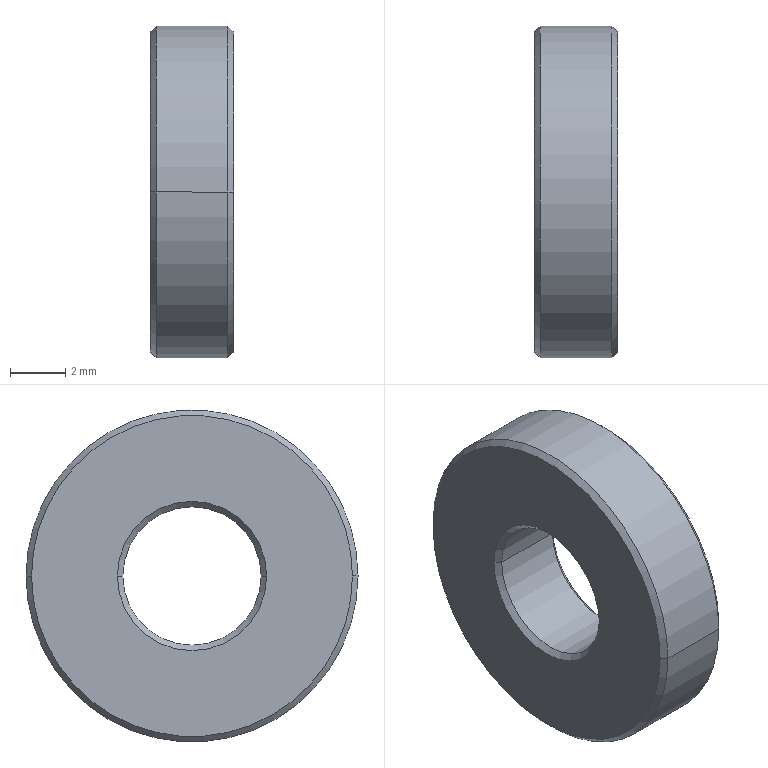Part | STEP file | WSSS12-5-3-16 | 1 solid | 14 faces | box 3 x 12 x 12 mm | volume 278.251 mm3 | cone 8 | cylinder 4 | plane 2 | commonest cylinder face diameters 5 x2 12 x2
STEP:
#1=CARTESIAN_POINT('',(0.,0.,0.));
#2=DIRECTION('',(0.,0.,1.));
#3=DIRECTION('',(1.,0.,0.));
#4=AXIS2_PLACEMENT_3D('',#1,#2,#3);
#5=CARTESIAN_POINT('',(2.8,-2.5,0.));
#6=VERTEX_POINT('',#5);
#7=CARTESIAN_POINT('',(0.2,-2.5,0.));
#8=VERTEX_POINT('',#7);
#9=CARTESIAN_POINT('',(-3.,-2.5,0.));
#10=DIRECTION('',(-1.,0.,0.));
#11=VECTOR('',#10,1.);
#12=LINE('',#9,#11);
#13=CARTESIAN_POINT('',(-3.,0.,0.));
#14=DIRECTION('',(-1.,0.,0.));
#15=DIRECTION('',(0.,-1.,0.));
#16=AXIS2_PLACEMENT_3D('',#13,#14,#15);
#17=CYLINDRICAL_SURFACE('',#16,2.5);
#18=CARTESIAN_POINT('',(6.283,0.));
#19=DIRECTION('',(0.,1.));
#20=VECTOR('',#19,1.);
#21=LINE('',#18,#20);
#22=(GEOMETRIC_REPRESENTATION_CONTEXT(2)PARAMETRIC_REPRESENTATION_CONTEXT()REPRESENTATION_CONTEXT('',''));
#23=DEFINITIONAL_REPRESENTATION('',(#21),#22);
#24=PCURVE('',#17,#23);
#25=CARTESIAN_POINT('',(-3.,0.,0.));
#26=DIRECTION('',(-1.,0.,0.));
#27=DIRECTION('',(0.,-1.,0.));
#28=AXIS2_PLACEMENT_3D('',#25,#26,#27);
#29=CYLINDRICAL_SURFACE('',#28,2.5);
#30=CARTESIAN_POINT('',(0.,0.));
#31=DIRECTION('',(0.,1.));
#32=VECTOR('',#31,1.);
#33=LINE('',#30,#32);
#34=(GEOMETRIC_REPRESENTATION_CONTEXT(2)PARAMETRIC_REPRESENTATION_CONTEXT()REPRESENTATION_CONTEXT('',''));
#35=DEFINITIONAL_REPRESENTATION('',(#33),#34);
#36=PCURVE('',#29,#35);
#37=SURFACE_CURVE('',#12,(#24,#36),.PCURVE_S1.);
#38=EDGE_CURVE('',#6,#8,#37,.T.);
#39=ORIENTED_EDGE('',*,*,#38,.T.);
#40=CARTESIAN_POINT('',(0.2,2.5,0.));
#41=VERTEX_POINT('',#40);
#42=CARTESIAN_POINT('',(0.2,0.,0.));
#43=DIRECTION('',(-1.,0.,0.));
#44=DIRECTION('',(0.,-1.,0.));
#45=AXIS2_PLACEMENT_3D('',#42,#43,#44);
#46=CIRCLE('',#45,2.5);
#47=CARTESIAN_POINT('',(0.,-3.2));
#48=DIRECTION('',(1.,0.));
#49=VECTOR('',#48,1.);
#50=LINE('',#47,#49);
#51=(GEOMETRIC_REPRESENTATION_CONTEXT(2)PARAMETRIC_REPRESENTATION_CONTEXT()REPRESENTATION_CONTEXT('',''));
#52=DEFINITIONAL_REPRESENTATION('',(#50),#51);
#53=PCURVE('',#17,#52);
#54=CARTESIAN_POINT('',(0.2,0.,0.));
#55=DIRECTION('',(-1.,0.,0.));
#56=DIRECTION('',(0.,-1.,0.));
#57=AXIS2_PLACEMENT_3D('',#54,#55,#56);
#58=CONICAL_SURFACE('',#57,2.5,0.7854);
#59=CARTESIAN_POINT('',(0.,0.));
#60=DIRECTION('',(1.,0.));
#61=VECTOR('',#60,1.);
#62=LINE('',#59,#61);
#63=(GEOMETRIC_REPRESENTATION_CONTEXT(2)PARAMETRIC_REPRESENTATION_CONTEXT()REPRESENTATION_CONTEXT('',''));
#64=DEFINITIONAL_REPRESENTATION('',(#62),#63);
#65=PCURVE('',#58,#64);
#66=SURFACE_CURVE('',#46,(#53,#65),.PCURVE_S1.);
#67=EDGE_CURVE('',#41,#8,#66,.T.);
#68=ORIENTED_EDGE('',*,*,#67,.F.);
#69=CARTESIAN_POINT('',(2.8,2.5,0.));
#70=VERTEX_POINT('',#69);
#71=CARTESIAN_POINT('',(-3.,2.5,0.));
#72=DIRECTION('',(-1.,0.,0.));
#73=VECTOR('',#72,1.);
#74=LINE('',#71,#73);
#75=CARTESIAN_POINT('',(3.142,0.));
#76=DIRECTION('',(0.,1.));
#77=VECTOR('',#76,1.);
#78=LINE('',#75,#77);
#79=(GEOMETRIC_REPRESENTATION_CONTEXT(2)PARAMETRIC_REPRESENTATION_CONTEXT()REPRESENTATION_CONTEXT('',''));
#80=DEFINITIONAL_REPRESENTATION('',(#78),#79);
#81=PCURVE('',#17,#80);
#82=CARTESIAN_POINT('',(3.142,0.));
#83=DIRECTION('',(0.,1.));
#84=VECTOR('',#83,1.);
#85=LINE('',#82,#84);
#86=(GEOMETRIC_REPRESENTATION_CONTEXT(2)PARAMETRIC_REPRESENTATION_CONTEXT()REPRESENTATION_CONTEXT('',''));
#87=DEFINITIONAL_REPRESENTATION('',(#85),#86);
#88=PCURVE('',#29,#87);
#89=SURFACE_CURVE('',#74,(#81,#88),.PCURVE_S1.);
#90=EDGE_CURVE('',#70,#41,#89,.T.);
#91=ORIENTED_EDGE('',*,*,#90,.F.);
#92=CARTESIAN_POINT('',(2.8,0.,0.));
#93=DIRECTION('',(-1.,0.,0.));
#94=DIRECTION('',(0.,-1.,0.));
#95=AXIS2_PLACEMENT_3D('',#92,#93,#94);
#96=CIRCLE('',#95,2.5);
#97=CARTESIAN_POINT('',(0.,-5.8));
#98=DIRECTION('',(1.,0.));
#99=VECTOR('',#98,1.);
#100=LINE('',#97,#99);
#101=(GEOMETRIC_REPRESENTATION_CONTEXT(2)PARAMETRIC_REPRESENTATION_CONTEXT()REPRESENTATION_CONTEXT('',''));
#102=DEFINITIONAL_REPRESENTATION('',(#100),#101);
#103=PCURVE('',#17,#102);
#104=CARTESIAN_POINT('',(3.,0.,0.));
#105=DIRECTION('',(1.,0.,0.));
#106=DIRECTION('',(0.,1.,0.));
#107=AXIS2_PLACEMENT_3D('',#104,#105,#106);
#108=CONICAL_SURFACE('',#107,2.7,0.7854);
#109=CARTESIAN_POINT('',(9.425,-0.2));
#110=DIRECTION('',(-1.,0.));
#111=VECTOR('',#110,1.);
#112=LINE('',#109,#111);
#113=(GEOMETRIC_REPRESENTATION_CONTEXT(2)PARAMETRIC_REPRESENTATION_CONTEXT()REPRESENTATION_CONTEXT('',''));
#114=DEFINITIONAL_REPRESENTATION('',(#112),#113);
#115=PCURVE('',#108,#114);
#116=SURFACE_CURVE('',#96,(#103,#115),.PCURVE_S1.);
#117=EDGE_CURVE('',#70,#6,#116,.T.);
#118=ORIENTED_EDGE('',*,*,#117,.T.);
#119=EDGE_LOOP('',(#39,#68,#91,#118));
#120=FACE_BOUND('',#119,.F.);
#121=ADVANCED_FACE('',(#120),#17,.F.);
#122=CARTESIAN_POINT('',(3.,2.7,0.));
#123=VERTEX_POINT('',#122);
#124=CARTESIAN_POINT('',(3.,2.7,0.));
#125=DIRECTION('',(0.7071,0.7071,0.));
#126=VECTOR('',#125,1.);
#127=LINE('',#124,#126);
#128=CARTESIAN_POINT('',(6.283,0.));
#129=DIRECTION('',(0.,1.));
#130=VECTOR('',#129,1.);
#131=LINE('',#128,#130);
#132=(GEOMETRIC_REPRESENTATION_CONTEXT(2)PARAMETRIC_REPRESENTATION_CONTEXT()REPRESENTATION_CONTEXT('',''));
#133=DEFINITIONAL_REPRESENTATION('',(#131),#132);
#134=PCURVE('',#108,#133);
#135=CARTESIAN_POINT('',(3.,0.,0.));
#136=DIRECTION('',(1.,0.,0.));
#137=DIRECTION('',(0.,1.,0.));
#138=AXIS2_PLACEMENT_3D('',#135,#136,#137);
#139=CONICAL_SURFACE('',#138,2.7,0.7854);
#140=CARTESIAN_POINT('',(0.,0.));
#141=DIRECTION('',(0.,1.));
#142=VECTOR('',#141,1.);
#143=LINE('',#140,#142);
#144=(GEOMETRIC_REPRESENTATION_CONTEXT(2)PARAMETRIC_REPRESENTATION_CONTEXT()REPRESENTATION_CONTEXT('',''));
#145=DEFINITIONAL_REPRESENTATION('',(#143),#144);
#146=PCURVE('',#139,#145);
#147=SURFACE_CURVE('',#127,(#134,#146),.PCURVE_S1.);
#148=EDGE_CURVE('',#70,#123,#147,.T.);
#149=ORIENTED_EDGE('',*,*,#148,.T.);
#150=CARTESIAN_POINT('',(3.,-2.7,0.));
#151=VERTEX_POINT('',#150);
#152=CARTESIAN_POINT('',(3.,0.,0.));
#153=DIRECTION('',(-1.,0.,0.));
#154=DIRECTION('',(0.,-1.,0.));
#155=AXIS2_PLACEMENT_3D('',#152,#153,#154);
#156=CIRCLE('',#155,2.7);
#157=CARTESIAN_POINT('',(9.425,0.));
#158=DIRECTION('',(-1.,0.));
#159=VECTOR('',#158,1.);
#160=LINE('',#157,#159);
#161=(GEOMETRIC_REPRESENTATION_CONTEXT(2)PARAMETRIC_REPRESENTATION_CONTEXT()REPRESENTATION_CONTEXT('',''));
#162=DEFINITIONAL_REPRESENTATION('',(#160),#161);
#163=PCURVE('',#108,#162);
#164=CARTESIAN_POINT('',(3.,-6.8,0.));
#165=DIRECTION('',(1.,0.,0.));
#166=DIRECTION('',(0.,1.,0.));
#167=AXIS2_PLACEMENT_3D('',#164,#165,#166);
#168=PLANE('',#167);
#169=CARTESIAN_POINT('',(4.1,0.));
#170=CARTESIAN_POINT('',(4.1,4.677));
#171=CARTESIAN_POINT('',(8.15,2.338));
#172=CARTESIAN_POINT('',(12.2,0.));
#173=CARTESIAN_POINT('',(8.15,-2.338));
#174=CARTESIAN_POINT('',(4.1,-4.677));
#175=CARTESIAN_POINT('',(4.1,0.));
#176=(BOUNDED_CURVE()B_SPLINE_CURVE(2,(#169,#170,#171,#172,#173,#174,#175),.UNSPECIFIED.,.T.,.F.)B_SPLINE_CURVE_WITH_KNOTS((1,2,2,2,2,1),(-2.094,0.,2.094,4.189,6.283,8.378),.UNSPECIFIED.)CURVE()GEOMETRIC_REPRESENTATION_ITEM()RATIONAL_B_SPLINE_CURVE((1.,0.5,1.,0.5,1.,0.5,1.))REPRESENTATION_ITEM(''));
#177=(GEOMETRIC_REPRESENTATION_CONTEXT(2)PARAMETRIC_REPRESENTATION_CONTEXT()REPRESENTATION_CONTEXT('',''));
#178=DEFINITIONAL_REPRESENTATION('',(#176),#177);
#179=PCURVE('',#168,#178);
#180=SURFACE_CURVE('',#156,(#163,#179),.PCURVE_S1.);
#181=EDGE_CURVE('',#123,#151,#180,.T.);
#182=ORIENTED_EDGE('',*,*,#181,.T.);
#183=CARTESIAN_POINT('',(3.,-2.7,0.));
#184=DIRECTION('',(0.7071,-0.7071,0.));
#185=VECTOR('',#184,1.);
#186=LINE('',#183,#185);
#187=CARTESIAN_POINT('',(3.142,0.));
#188=DIRECTION('',(0.,1.));
#189=VECTOR('',#188,1.);
#190=LINE('',#187,#189);
#191=(GEOMETRIC_REPRESENTATION_CONTEXT(2)PARAMETRIC_REPRESENTATION_CONTEXT()REPRESENTATION_CONTEXT('',''));
#192=DEFINITIONAL_REPRESENTATION('',(#190),#191);
#193=PCURVE('',#108,#192);
#194=CARTESIAN_POINT('',(3.142,0.));
#195=DIRECTION('',(0.,1.));
#196=VECTOR('',#195,1.);
#197=LINE('',#194,#196);
#198=(GEOMETRIC_REPRESENTATION_CONTEXT(2)PARAMETRIC_REPRESENTATION_CONTEXT()REPRESENTATION_CONTEXT('',''));
#199=DEFINITIONAL_REPRESENTATION('',(#197),#198);
#200=PCURVE('',#139,#199);
#201=SURFACE_CURVE('',#186,(#193,#200),.PCURVE_S1.);
#202=EDGE_CURVE('',#6,#151,#201,.T.);
#203=ORIENTED_EDGE('',*,*,#202,.F.);
#204=ORIENTED_EDGE('',*,*,#117,.F.);
#205=EDGE_LOOP('',(#149,#182,#203,#204));
#206=FACE_BOUND('',#205,.F.);
#207=ADVANCED_FACE('',(#206),#108,.F.);
#208=CARTESIAN_POINT('',(3.,-5.8,0.));
#209=VERTEX_POINT('',#208);
#210=CARTESIAN_POINT('',(3.,5.8,0.));
#211=VERTEX_POINT('',#210);
#212=CARTESIAN_POINT('',(3.,0.,0.));
#213=DIRECTION('',(-1.,0.,0.));
#214=DIRECTION('',(0.,1.,0.));
#215=AXIS2_PLACEMENT_3D('',#212,#213,#214);
#216=CIRCLE('',#215,5.8);
#217=CARTESIAN_POINT('',(2.8,0.,0.));
#218=DIRECTION('',(-1.,0.,0.));
#219=DIRECTION('',(0.,-1.,0.));
#220=AXIS2_PLACEMENT_3D('',#217,#218,#219);
#221=CONICAL_SURFACE('',#220,6.,0.7854);
#222=CARTESIAN_POINT('',(-3.142,-0.2));
#223=DIRECTION('',(1.,0.));
#224=VECTOR('',#223,1.);
#225=LINE('',#222,#224);
#226=(GEOMETRIC_REPRESENTATION_CONTEXT(2)PARAMETRIC_REPRESENTATION_CONTEXT()REPRESENTATION_CONTEXT('',''));
#227=DEFINITIONAL_REPRESENTATION('',(#225),#226);
#228=PCURVE('',#221,#227);
#229=CARTESIAN_POINT('',(12.6,0.));
#230=CARTESIAN_POINT('',(12.6,-10.046));
#231=CARTESIAN_POINT('',(3.9,-5.023));
#232=CARTESIAN_POINT('',(-4.8,0.));
#233=CARTESIAN_POINT('',(3.9,5.023));
#234=CARTESIAN_POINT('',(12.6,10.046));
#235=CARTESIAN_POINT('',(12.6,0.));
#236=(BOUNDED_CURVE()B_SPLINE_CURVE(2,(#229,#230,#231,#232,#233,#234,#235),.UNSPECIFIED.,.T.,.F.)B_SPLINE_CURVE_WITH_KNOTS((1,2,2,2,2,1),(-2.094,0.,2.094,4.189,6.283,8.378),.UNSPECIFIED.)CURVE()GEOMETRIC_REPRESENTATION_ITEM()RATIONAL_B_SPLINE_CURVE((1.,0.5,1.,0.5,1.,0.5,1.))REPRESENTATION_ITEM(''));
#237=(GEOMETRIC_REPRESENTATION_CONTEXT(2)PARAMETRIC_REPRESENTATION_CONTEXT()REPRESENTATION_CONTEXT('',''));
#238=DEFINITIONAL_REPRESENTATION('',(#236),#237);
#239=PCURVE('',#168,#238);
#240=SURFACE_CURVE('',#216,(#228,#239),.PCURVE_S1.);
#241=EDGE_CURVE('',#209,#211,#240,.T.);
#242=ORIENTED_EDGE('',*,*,#241,.T.);
#243=CARTESIAN_POINT('',(2.8,6.,0.));
#244=VERTEX_POINT('',#243);
#245=CARTESIAN_POINT('',(2.8,6.,0.));
#246=DIRECTION('',(-0.7071,0.7071,0.));
#247=VECTOR('',#246,1.);
#248=LINE('',#245,#247);
#249=CARTESIAN_POINT('',(3.142,0.));
#250=DIRECTION('',(0.,1.));
#251=VECTOR('',#250,1.);
#252=LINE('',#249,#251);
#253=(GEOMETRIC_REPRESENTATION_CONTEXT(2)PARAMETRIC_REPRESENTATION_CONTEXT()REPRESENTATION_CONTEXT('',''));
#254=DEFINITIONAL_REPRESENTATION('',(#252),#253);
#255=PCURVE('',#221,#254);
#256=CARTESIAN_POINT('',(2.8,0.,0.));
#257=DIRECTION('',(-1.,0.,0.));
#258=DIRECTION('',(0.,-1.,0.));
#259=AXIS2_PLACEMENT_3D('',#256,#257,#258);
#260=CONICAL_SURFACE('',#259,6.,0.7854);
#261=CARTESIAN_POINT('',(3.142,0.));
#262=DIRECTION('',(0.,1.));
#263=VECTOR('',#262,1.);
#264=LINE('',#261,#263);
#265=(GEOMETRIC_REPRESENTATION_CONTEXT(2)PARAMETRIC_REPRESENTATION_CONTEXT()REPRESENTATION_CONTEXT('',''));
#266=DEFINITIONAL_REPRESENTATION('',(#264),#265);
#267=PCURVE('',#260,#266);
#268=SURFACE_CURVE('',#248,(#255,#267),.PCURVE_S1.);
#269=EDGE_CURVE('',#211,#244,#268,.T.);
#270=ORIENTED_EDGE('',*,*,#269,.T.);
#271=CARTESIAN_POINT('',(2.8,-6.,0.));
#272=VERTEX_POINT('',#271);
#273=CARTESIAN_POINT('',(2.8,0.,0.));
#274=DIRECTION('',(-1.,0.,0.));
#275=DIRECTION('',(0.,-1.,0.));
#276=AXIS2_PLACEMENT_3D('',#273,#274,#275);
#277=CIRCLE('',#276,6.);
#278=CARTESIAN_POINT('',(0.,0.));
#279=DIRECTION('',(1.,0.));
#280=VECTOR('',#279,1.);
#281=LINE('',#278,#280);
#282=(GEOMETRIC_REPRESENTATION_CONTEXT(2)PARAMETRIC_REPRESENTATION_CONTEXT()REPRESENTATION_CONTEXT('',''));
#283=DEFINITIONAL_REPRESENTATION('',(#281),#282);
#284=PCURVE('',#221,#283);
#285=CARTESIAN_POINT('',(-3.,0.,0.));
#286=DIRECTION('',(-1.,0.,0.));
#287=DIRECTION('',(0.,-1.,0.));
#288=AXIS2_PLACEMENT_3D('',#285,#286,#287);
#289=CYLINDRICAL_SURFACE('',#288,6.);
#290=CARTESIAN_POINT('',(0.,-5.8));
#291=DIRECTION('',(1.,0.));
#292=VECTOR('',#291,1.);
#293=LINE('',#290,#292);
#294=(GEOMETRIC_REPRESENTATION_CONTEXT(2)PARAMETRIC_REPRESENTATION_CONTEXT()REPRESENTATION_CONTEXT('',''));
#295=DEFINITIONAL_REPRESENTATION('',(#293),#294);
#296=PCURVE('',#289,#295);
#297=SURFACE_CURVE('',#277,(#284,#296),.PCURVE_S1.);
#298=EDGE_CURVE('',#272,#244,#297,.T.);
#299=ORIENTED_EDGE('',*,*,#298,.F.);
#300=CARTESIAN_POINT('',(2.8,-6.,0.));
#301=DIRECTION('',(-0.7071,-0.7071,0.));
#302=VECTOR('',#301,1.);
#303=LINE('',#300,#302);
#304=CARTESIAN_POINT('',(0.,0.));
#305=DIRECTION('',(0.,1.));
#306=VECTOR('',#305,1.);
#307=LINE('',#304,#306);
#308=(GEOMETRIC_REPRESENTATION_CONTEXT(2)PARAMETRIC_REPRESENTATION_CONTEXT()REPRESENTATION_CONTEXT('',''));
#309=DEFINITIONAL_REPRESENTATION('',(#307),#308);
#310=PCURVE('',#221,#309);
#311=CARTESIAN_POINT('',(6.283,0.));
#312=DIRECTION('',(0.,1.));
#313=VECTOR('',#312,1.);
#314=LINE('',#311,#313);
#315=(GEOMETRIC_REPRESENTATION_CONTEXT(2)PARAMETRIC_REPRESENTATION_CONTEXT()REPRESENTATION_CONTEXT('',''));
#316=DEFINITIONAL_REPRESENTATION('',(#314),#315);
#317=PCURVE('',#260,#316);
#318=SURFACE_CURVE('',#303,(#310,#317),.PCURVE_S1.);
#319=EDGE_CURVE('',#209,#272,#318,.T.);
#320=ORIENTED_EDGE('',*,*,#319,.F.);
#321=EDGE_LOOP('',(#242,#270,#299,#320));
#322=FACE_BOUND('',#321,.T.);
#323=ADVANCED_FACE('',(#322),#221,.T.);
#324=ORIENTED_EDGE('',*,*,#298,.T.);
#325=CARTESIAN_POINT('',(0.2,6.,0.));
#326=VERTEX_POINT('',#325);
#327=CARTESIAN_POINT('',(-3.,6.,0.));
#328=DIRECTION('',(-1.,0.,0.));
#329=VECTOR('',#328,1.);
#330=LINE('',#327,#329);
#331=CARTESIAN_POINT('',(3.142,0.));
#332=DIRECTION('',(0.,1.));
#333=VECTOR('',#332,1.);
#334=LINE('',#331,#333);
#335=(GEOMETRIC_REPRESENTATION_CONTEXT(2)PARAMETRIC_REPRESENTATION_CONTEXT()REPRESENTATION_CONTEXT('',''));
#336=DEFINITIONAL_REPRESENTATION('',(#334),#335);
#337=PCURVE('',#289,#336);
#338=CARTESIAN_POINT('',(-3.,0.,0.));
#339=DIRECTION('',(-1.,0.,0.));
#340=DIRECTION('',(0.,-1.,0.));
#341=AXIS2_PLACEMENT_3D('',#338,#339,#340);
#342=CYLINDRICAL_SURFACE('',#341,6.);
#343=CARTESIAN_POINT('',(3.142,0.));
#344=DIRECTION('',(0.,1.));
#345=VECTOR('',#344,1.);
#346=LINE('',#343,#345);
#347=(GEOMETRIC_REPRESENTATION_CONTEXT(2)PARAMETRIC_REPRESENTATION_CONTEXT()REPRESENTATION_CONTEXT('',''));
#348=DEFINITIONAL_REPRESENTATION('',(#346),#347);
#349=PCURVE('',#342,#348);
#350=SURFACE_CURVE('',#330,(#337,#349),.PCURVE_S1.);
#351=EDGE_CURVE('',#244,#326,#350,.T.);
#352=ORIENTED_EDGE('',*,*,#351,.T.);
#353=CARTESIAN_POINT('',(0.2,-6.,0.));
#354=VERTEX_POINT('',#353);
#355=CARTESIAN_POINT('',(0.2,0.,0.));
#356=DIRECTION('',(-1.,0.,0.));
#357=DIRECTION('',(0.,1.,0.));
#358=AXIS2_PLACEMENT_3D('',#355,#356,#357);
#359=CIRCLE('',#358,6.);
#360=CARTESIAN_POINT('',(-3.142,-3.2));
#361=DIRECTION('',(1.,0.));
#362=VECTOR('',#361,1.);
#363=LINE('',#360,#362);
#364=(GEOMETRIC_REPRESENTATION_CONTEXT(2)PARAMETRIC_REPRESENTATION_CONTEXT()REPRESENTATION_CONTEXT('',''));
#365=DEFINITIONAL_REPRESENTATION('',(#363),#364);
#366=PCURVE('',#289,#365);
#367=CARTESIAN_POINT('',(0.,0.,0.));
#368=DIRECTION('',(1.,0.,0.));
#369=DIRECTION('',(0.,1.,0.));
#370=AXIS2_PLACEMENT_3D('',#367,#368,#369);
#371=CONICAL_SURFACE('',#370,5.8,0.7854);
#372=CARTESIAN_POINT('',(6.283,0.2));
#373=DIRECTION('',(-1.,0.));
#374=VECTOR('',#373,1.);
#375=LINE('',#372,#374);
#376=(GEOMETRIC_REPRESENTATION_CONTEXT(2)PARAMETRIC_REPRESENTATION_CONTEXT()REPRESENTATION_CONTEXT('',''));
#377=DEFINITIONAL_REPRESENTATION('',(#375),#376);
#378=PCURVE('',#371,#377);
#379=SURFACE_CURVE('',#359,(#366,#378),.PCURVE_S1.);
#380=EDGE_CURVE('',#354,#326,#379,.T.);
#381=ORIENTED_EDGE('',*,*,#380,.F.);
#382=CARTESIAN_POINT('',(-3.,-6.,0.));
#383=DIRECTION('',(-1.,0.,0.));
#384=VECTOR('',#383,1.);
#385=LINE('',#382,#384);
#386=CARTESIAN_POINT('',(0.,0.));
#387=DIRECTION('',(0.,1.));
#388=VECTOR('',#387,1.);
#389=LINE('',#386,#388);
#390=(GEOMETRIC_REPRESENTATION_CONTEXT(2)PARAMETRIC_REPRESENTATION_CONTEXT()REPRESENTATION_CONTEXT('',''));
#391=DEFINITIONAL_REPRESENTATION('',(#389),#390);
#392=PCURVE('',#289,#391);
#393=CARTESIAN_POINT('',(6.283,0.));
#394=DIRECTION('',(0.,1.));
#395=VECTOR('',#394,1.);
#396=LINE('',#393,#395);
#397=(GEOMETRIC_REPRESENTATION_CONTEXT(2)PARAMETRIC_REPRESENTATION_CONTEXT()REPRESENTATION_CONTEXT('',''));
#398=DEFINITIONAL_REPRESENTATION('',(#396),#397);
#399=PCURVE('',#342,#398);
#400=SURFACE_CURVE('',#385,(#392,#399),.PCURVE_S1.);
#401=EDGE_CURVE('',#272,#354,#400,.T.);
#402=ORIENTED_EDGE('',*,*,#401,.F.);
#403=EDGE_LOOP('',(#324,#352,#381,#402));
#404=FACE_BOUND('',#403,.T.);
#405=ADVANCED_FACE('',(#404),#289,.T.);
#406=CARTESIAN_POINT('',(0.,-5.8,0.));
#407=VERTEX_POINT('',#406);
#408=CARTESIAN_POINT('',(0.,5.8,0.));
#409=VERTEX_POINT('',#408);
#410=CARTESIAN_POINT('',(0.,0.,0.));
#411=DIRECTION('',(-1.,0.,0.));
#412=DIRECTION('',(0.,-1.,0.));
#413=AXIS2_PLACEMENT_3D('',#410,#411,#412);
#414=CIRCLE('',#413,5.8);
#415=CARTESIAN_POINT('',(3.142,0.));
#416=DIRECTION('',(-1.,0.));
#417=VECTOR('',#416,1.);
#418=LINE('',#415,#417);
#419=(GEOMETRIC_REPRESENTATION_CONTEXT(2)PARAMETRIC_REPRESENTATION_CONTEXT()REPRESENTATION_CONTEXT('',''));
#420=DEFINITIONAL_REPRESENTATION('',(#418),#419);
#421=PCURVE('',#371,#420);
#422=CARTESIAN_POINT('',(0.,-2.7,0.));
#423=DIRECTION('',(-1.,0.,0.));
#424=DIRECTION('',(0.,-1.,0.));
#425=AXIS2_PLACEMENT_3D('',#422,#423,#424);
#426=PLANE('',#425);
#427=CARTESIAN_POINT('',(-2.7,0.));
#428=DIRECTION('',(1.,0.));
#429=AXIS2_PLACEMENT_2D('',#427,#428);
#430=CIRCLE('',#429,5.8);
#431=(GEOMETRIC_REPRESENTATION_CONTEXT(2)PARAMETRIC_REPRESENTATION_CONTEXT()REPRESENTATION_CONTEXT('',''));
#432=DEFINITIONAL_REPRESENTATION('',(#430),#431);
#433=PCURVE('',#426,#432);
#434=SURFACE_CURVE('',#414,(#421,#433),.PCURVE_S1.);
#435=EDGE_CURVE('',#407,#409,#434,.T.);
#436=ORIENTED_EDGE('',*,*,#435,.F.);
#437=CARTESIAN_POINT('',(0.,-5.8,0.));
#438=DIRECTION('',(0.7071,-0.7071,0.));
#439=VECTOR('',#438,1.);
#440=LINE('',#437,#439);
#441=CARTESIAN_POINT('',(3.142,0.));
#442=DIRECTION('',(0.,1.));
#443=VECTOR('',#442,1.);
#444=LINE('',#441,#443);
#445=(GEOMETRIC_REPRESENTATION_CONTEXT(2)PARAMETRIC_REPRESENTATION_CONTEXT()REPRESENTATION_CONTEXT('',''));
#446=DEFINITIONAL_REPRESENTATION('',(#444),#445);
#447=PCURVE('',#371,#446);
#448=CARTESIAN_POINT('',(0.,0.,0.));
#449=DIRECTION('',(1.,0.,0.));
#450=DIRECTION('',(0.,1.,0.));
#451=AXIS2_PLACEMENT_3D('',#448,#449,#450);
#452=CONICAL_SURFACE('',#451,5.8,0.7854);
#453=CARTESIAN_POINT('',(3.142,0.));
#454=DIRECTION('',(0.,1.));
#455=VECTOR('',#454,1.);
#456=LINE('',#453,#455);
#457=(GEOMETRIC_REPRESENTATION_CONTEXT(2)PARAMETRIC_REPRESENTATION_CONTEXT()REPRESENTATION_CONTEXT('',''));
#458=DEFINITIONAL_REPRESENTATION('',(#456),#457);
#459=PCURVE('',#452,#458);
#460=SURFACE_CURVE('',#440,(#447,#459),.PCURVE_S1.);
#461=EDGE_CURVE('',#407,#354,#460,.T.);
#462=ORIENTED_EDGE('',*,*,#461,.T.);
#463=ORIENTED_EDGE('',*,*,#380,.T.);
#464=CARTESIAN_POINT('',(0.,5.8,0.));
#465=DIRECTION('',(0.7071,0.7071,0.));
#466=VECTOR('',#465,1.);
#467=LINE('',#464,#466);
#468=CARTESIAN_POINT('',(0.,0.));
#469=DIRECTION('',(0.,1.));
#470=VECTOR('',#469,1.);
#471=LINE('',#468,#470);
#472=(GEOMETRIC_REPRESENTATION_CONTEXT(2)PARAMETRIC_REPRESENTATION_CONTEXT()REPRESENTATION_CONTEXT('',''));
#473=DEFINITIONAL_REPRESENTATION('',(#471),#472);
#474=PCURVE('',#371,#473);
#475=CARTESIAN_POINT('',(6.283,0.));
#476=DIRECTION('',(0.,1.));
#477=VECTOR('',#476,1.);
#478=LINE('',#475,#477);
#479=(GEOMETRIC_REPRESENTATION_CONTEXT(2)PARAMETRIC_REPRESENTATION_CONTEXT()REPRESENTATION_CONTEXT('',''));
#480=DEFINITIONAL_REPRESENTATION('',(#478),#479);
#481=PCURVE('',#452,#480);
#482=SURFACE_CURVE('',#467,(#474,#481),.PCURVE_S1.);
#483=EDGE_CURVE('',#409,#326,#482,.T.);
#484=ORIENTED_EDGE('',*,*,#483,.F.);
#485=EDGE_LOOP('',(#436,#462,#463,#484));
#486=FACE_BOUND('',#485,.T.);
#487=ADVANCED_FACE('',(#486),#371,.T.);
#488=CARTESIAN_POINT('',(0.,-2.7,0.));
#489=VERTEX_POINT('',#488);
#490=CARTESIAN_POINT('',(0.2,-2.5,0.));
#491=DIRECTION('',(-0.7071,-0.7071,0.));
#492=VECTOR('',#491,1.);
#493=LINE('',#490,#492);
#494=CARTESIAN_POINT('',(6.283,0.));
#495=DIRECTION('',(0.,1.));
#496=VECTOR('',#495,1.);
#497=LINE('',#494,#496);
#498=(GEOMETRIC_REPRESENTATION_CONTEXT(2)PARAMETRIC_REPRESENTATION_CONTEXT()REPRESENTATION_CONTEXT('',''));
#499=DEFINITIONAL_REPRESENTATION('',(#497),#498);
#500=PCURVE('',#58,#499);
#501=CARTESIAN_POINT('',(0.2,0.,0.));
#502=DIRECTION('',(-1.,0.,0.));
#503=DIRECTION('',(0.,-1.,0.));
#504=AXIS2_PLACEMENT_3D('',#501,#502,#503);
#505=CONICAL_SURFACE('',#504,2.5,0.7854);
#506=CARTESIAN_POINT('',(0.,0.));
#507=DIRECTION('',(0.,1.));
#508=VECTOR('',#507,1.);
#509=LINE('',#506,#508);
#510=(GEOMETRIC_REPRESENTATION_CONTEXT(2)PARAMETRIC_REPRESENTATION_CONTEXT()REPRESENTATION_CONTEXT('',''));
#511=DEFINITIONAL_REPRESENTATION('',(#509),#510);
#512=PCURVE('',#505,#511);
#513=SURFACE_CURVE('',#493,(#500,#512),.PCURVE_S1.);
#514=EDGE_CURVE('',#8,#489,#513,.T.);
#515=ORIENTED_EDGE('',*,*,#514,.T.);
#516=CARTESIAN_POINT('',(0.,2.7,0.));
#517=VERTEX_POINT('',#516);
#518=CARTESIAN_POINT('',(0.,0.,0.));
#519=DIRECTION('',(-1.,0.,0.));
#520=DIRECTION('',(0.,-1.,0.));
#521=AXIS2_PLACEMENT_3D('',#518,#519,#520);
#522=CIRCLE('',#521,2.7);
#523=CARTESIAN_POINT('',(0.,0.2));
#524=DIRECTION('',(1.,0.));
#525=VECTOR('',#524,1.);
#526=LINE('',#523,#525);
#527=(GEOMETRIC_REPRESENTATION_CONTEXT(2)PARAMETRIC_REPRESENTATION_CONTEXT()REPRESENTATION_CONTEXT('',''));
#528=DEFINITIONAL_REPRESENTATION('',(#526),#527);
#529=PCURVE('',#58,#528);
#530=CARTESIAN_POINT('',(-2.7,0.));
#531=DIRECTION('',(1.,0.));
#532=AXIS2_PLACEMENT_2D('',#530,#531);
#533=CIRCLE('',#532,2.7);
#534=(GEOMETRIC_REPRESENTATION_CONTEXT(2)PARAMETRIC_REPRESENTATION_CONTEXT()REPRESENTATION_CONTEXT('',''));
#535=DEFINITIONAL_REPRESENTATION('',(#533),#534);
#536=PCURVE('',#426,#535);
#537=SURFACE_CURVE('',#522,(#529,#536),.PCURVE_S1.);
#538=EDGE_CURVE('',#517,#489,#537,.T.);
#539=ORIENTED_EDGE('',*,*,#538,.F.);
#540=CARTESIAN_POINT('',(0.2,2.5,0.));
#541=DIRECTION('',(-0.7071,0.7071,0.));
#542=VECTOR('',#541,1.);
#543=LINE('',#540,#542);
#544=CARTESIAN_POINT('',(3.142,0.));
#545=DIRECTION('',(0.,1.));
#546=VECTOR('',#545,1.);
#547=LINE('',#544,#546);
#548=(GEOMETRIC_REPRESENTATION_CONTEXT(2)PARAMETRIC_REPRESENTATION_CONTEXT()REPRESENTATION_CONTEXT('',''));
#549=DEFINITIONAL_REPRESENTATION('',(#547),#548);
#550=PCURVE('',#58,#549);
#551=CARTESIAN_POINT('',(3.142,0.));
#552=DIRECTION('',(0.,1.));
#553=VECTOR('',#552,1.);
#554=LINE('',#551,#553);
#555=(GEOMETRIC_REPRESENTATION_CONTEXT(2)PARAMETRIC_REPRESENTATION_CONTEXT()REPRESENTATION_CONTEXT('',''));
#556=DEFINITIONAL_REPRESENTATION('',(#554),#555);
#557=PCURVE('',#505,#556);
#558=SURFACE_CURVE('',#543,(#550,#557),.PCURVE_S1.);
#559=EDGE_CURVE('',#41,#517,#558,.T.);
#560=ORIENTED_EDGE('',*,*,#559,.F.);
#561=ORIENTED_EDGE('',*,*,#67,.T.);
#562=EDGE_LOOP('',(#515,#539,#560,#561));
#563=FACE_BOUND('',#562,.F.);
#564=ADVANCED_FACE('',(#563),#58,.F.);
#565=CARTESIAN_POINT('',(0.,0.,0.));
#566=DIRECTION('',(-1.,0.,0.));
#567=DIRECTION('',(0.,-1.,0.));
#568=AXIS2_PLACEMENT_3D('',#565,#566,#567);
#569=CIRCLE('',#568,2.7);
#570=CARTESIAN_POINT('',(0.,0.2));
#571=DIRECTION('',(1.,0.));
#572=VECTOR('',#571,1.);
#573=LINE('',#570,#572);
#574=(GEOMETRIC_REPRESENTATION_CONTEXT(2)PARAMETRIC_REPRESENTATION_CONTEXT()REPRESENTATION_CONTEXT('',''));
#575=DEFINITIONAL_REPRESENTATION('',(#573),#574);
#576=PCURVE('',#505,#575);
#577=CARTESIAN_POINT('',(-2.7,0.));
#578=DIRECTION('',(1.,0.));
#579=AXIS2_PLACEMENT_2D('',#577,#578);
#580=CIRCLE('',#579,2.7);
#581=(GEOMETRIC_REPRESENTATION_CONTEXT(2)PARAMETRIC_REPRESENTATION_CONTEXT()REPRESENTATION_CONTEXT('',''));
#582=DEFINITIONAL_REPRESENTATION('',(#580),#581);
#583=PCURVE('',#426,#582);
#584=SURFACE_CURVE('',#569,(#576,#583),.PCURVE_S1.);
#585=EDGE_CURVE('',#489,#517,#584,.T.);
#586=ORIENTED_EDGE('',*,*,#585,.F.);
#587=ORIENTED_EDGE('',*,*,#514,.F.);
#588=CARTESIAN_POINT('',(0.2,0.,0.));
#589=DIRECTION('',(-1.,0.,0.));
#590=DIRECTION('',(0.,-1.,0.));
#591=AXIS2_PLACEMENT_3D('',#588,#589,#590);
#592=CIRCLE('',#591,2.5);
#593=CARTESIAN_POINT('',(0.,0.));
#594=DIRECTION('',(1.,0.));
#595=VECTOR('',#594,1.);
#596=LINE('',#593,#595);
#597=(GEOMETRIC_REPRESENTATION_CONTEXT(2)PARAMETRIC_REPRESENTATION_CONTEXT()REPRESENTATION_CONTEXT('',''));
#598=DEFINITIONAL_REPRESENTATION('',(#596),#597);
#599=PCURVE('',#505,#598);
#600=CARTESIAN_POINT('',(0.,-3.2));
#601=DIRECTION('',(1.,0.));
#602=VECTOR('',#601,1.);
#603=LINE('',#600,#602);
#604=(GEOMETRIC_REPRESENTATION_CONTEXT(2)PARAMETRIC_REPRESENTATION_CONTEXT()REPRESENTATION_CONTEXT('',''));
#605=DEFINITIONAL_REPRESENTATION('',(#603),#604);
#606=PCURVE('',#29,#605);
#607=SURFACE_CURVE('',#592,(#599,#606),.PCURVE_S1.);
#608=EDGE_CURVE('',#8,#41,#607,.T.);
#609=ORIENTED_EDGE('',*,*,#608,.T.);
#610=ORIENTED_EDGE('',*,*,#559,.T.);
#611=EDGE_LOOP('',(#586,#587,#609,#610));
#612=FACE_BOUND('',#611,.F.);
#613=ADVANCED_FACE('',(#612),#505,.F.);
#614=CARTESIAN_POINT('',(0.,0.,0.));
#615=DIRECTION('',(-1.,0.,0.));
#616=DIRECTION('',(0.,-1.,0.));
#617=AXIS2_PLACEMENT_3D('',#614,#615,#616);
#618=CIRCLE('',#617,5.8);
#619=CARTESIAN_POINT('',(-2.7,0.));
#620=DIRECTION('',(1.,0.));
#621=AXIS2_PLACEMENT_2D('',#619,#620);
#622=CIRCLE('',#621,5.8);
#623=(GEOMETRIC_REPRESENTATION_CONTEXT(2)PARAMETRIC_REPRESENTATION_CONTEXT()REPRESENTATION_CONTEXT('',''));
#624=DEFINITIONAL_REPRESENTATION('',(#622),#623);
#625=PCURVE('',#426,#624);
#626=CARTESIAN_POINT('',(9.425,0.));
#627=DIRECTION('',(-1.,0.));
#628=VECTOR('',#627,1.);
#629=LINE('',#626,#628);
#630=(GEOMETRIC_REPRESENTATION_CONTEXT(2)PARAMETRIC_REPRESENTATION_CONTEXT()REPRESENTATION_CONTEXT('',''));
#631=DEFINITIONAL_REPRESENTATION('',(#629),#630);
#632=PCURVE('',#452,#631);
#633=SURFACE_CURVE('',#618,(#625,#632),.PCURVE_S1.);
#634=EDGE_CURVE('',#409,#407,#633,.T.);
#635=ORIENTED_EDGE('',*,*,#634,.T.);
#636=ORIENTED_EDGE('',*,*,#435,.T.);
#637=EDGE_LOOP('',(#635,#636));
#638=FACE_BOUND('',#637,.T.);
#639=ORIENTED_EDGE('',*,*,#585,.F.);
#640=ORIENTED_EDGE('',*,*,#538,.F.);
#641=EDGE_LOOP('',(#639,#640));
#642=FACE_BOUND('',#641,.T.);
#643=ADVANCED_FACE('',(#638,#642),#426,.T.);
#644=ORIENTED_EDGE('',*,*,#461,.F.);
#645=ORIENTED_EDGE('',*,*,#634,.F.);
#646=ORIENTED_EDGE('',*,*,#483,.T.);
#647=CARTESIAN_POINT('',(0.2,0.,0.));
#648=DIRECTION('',(-1.,0.,0.));
#649=DIRECTION('',(0.,1.,0.));
#650=AXIS2_PLACEMENT_3D('',#647,#648,#649);
#651=CIRCLE('',#650,6.);
#652=CARTESIAN_POINT('',(6.283,0.2));
#653=DIRECTION('',(-1.,0.));
#654=VECTOR('',#653,1.);
#655=LINE('',#652,#654);
#656=(GEOMETRIC_REPRESENTATION_CONTEXT(2)PARAMETRIC_REPRESENTATION_CONTEXT()REPRESENTATION_CONTEXT('',''));
#657=DEFINITIONAL_REPRESENTATION('',(#655),#656);
#658=PCURVE('',#452,#657);
#659=CARTESIAN_POINT('',(3.142,-3.2));
#660=DIRECTION('',(1.,0.));
#661=VECTOR('',#660,1.);
#662=LINE('',#659,#661);
#663=(GEOMETRIC_REPRESENTATION_CONTEXT(2)PARAMETRIC_REPRESENTATION_CONTEXT()REPRESENTATION_CONTEXT('',''));
#664=DEFINITIONAL_REPRESENTATION('',(#662),#663);
#665=PCURVE('',#342,#664);
#666=SURFACE_CURVE('',#651,(#658,#665),.PCURVE_S1.);
#667=EDGE_CURVE('',#326,#354,#666,.T.);
#668=ORIENTED_EDGE('',*,*,#667,.T.);
#669=EDGE_LOOP('',(#644,#645,#646,#668));
#670=FACE_BOUND('',#669,.T.);
#671=ADVANCED_FACE('',(#670),#452,.T.);
#672=ORIENTED_EDGE('',*,*,#351,.F.);
#673=CARTESIAN_POINT('',(2.8,0.,0.));
#674=DIRECTION('',(-1.,0.,0.));
#675=DIRECTION('',(0.,-1.,0.));
#676=AXIS2_PLACEMENT_3D('',#673,#674,#675);
#677=CIRCLE('',#676,6.);
#678=CARTESIAN_POINT('',(0.,-5.8));
#679=DIRECTION('',(1.,0.));
#680=VECTOR('',#679,1.);
#681=LINE('',#678,#680);
#682=(GEOMETRIC_REPRESENTATION_CONTEXT(2)PARAMETRIC_REPRESENTATION_CONTEXT()REPRESENTATION_CONTEXT('',''));
#683=DEFINITIONAL_REPRESENTATION('',(#681),#682);
#684=PCURVE('',#342,#683);
#685=CARTESIAN_POINT('',(0.,0.));
#686=DIRECTION('',(1.,0.));
#687=VECTOR('',#686,1.);
#688=LINE('',#685,#687);
#689=(GEOMETRIC_REPRESENTATION_CONTEXT(2)PARAMETRIC_REPRESENTATION_CONTEXT()REPRESENTATION_CONTEXT('',''));
#690=DEFINITIONAL_REPRESENTATION('',(#688),#689);
#691=PCURVE('',#260,#690);
#692=SURFACE_CURVE('',#677,(#684,#691),.PCURVE_S1.);
#693=EDGE_CURVE('',#244,#272,#692,.T.);
#694=ORIENTED_EDGE('',*,*,#693,.T.);
#695=ORIENTED_EDGE('',*,*,#401,.T.);
#696=ORIENTED_EDGE('',*,*,#667,.F.);
#697=EDGE_LOOP('',(#672,#694,#695,#696));
#698=FACE_BOUND('',#697,.T.);
#699=ADVANCED_FACE('',(#698),#342,.T.);
#700=ORIENTED_EDGE('',*,*,#269,.F.);
#701=CARTESIAN_POINT('',(3.,0.,0.));
#702=DIRECTION('',(-1.,0.,0.));
#703=DIRECTION('',(0.,1.,0.));
#704=AXIS2_PLACEMENT_3D('',#701,#702,#703);
#705=CIRCLE('',#704,5.8);
#706=CARTESIAN_POINT('',(3.142,-0.2));
#707=DIRECTION('',(1.,0.));
#708=VECTOR('',#707,1.);
#709=LINE('',#706,#708);
#710=(GEOMETRIC_REPRESENTATION_CONTEXT(2)PARAMETRIC_REPRESENTATION_CONTEXT()REPRESENTATION_CONTEXT('',''));
#711=DEFINITIONAL_REPRESENTATION('',(#709),#710);
#712=PCURVE('',#260,#711);
#713=CARTESIAN_POINT('',(12.6,0.));
#714=CARTESIAN_POINT('',(12.6,-10.046));
#715=CARTESIAN_POINT('',(3.9,-5.023));
#716=CARTESIAN_POINT('',(-4.8,0.));
#717=CARTESIAN_POINT('',(3.9,5.023));
#718=CARTESIAN_POINT('',(12.6,10.046));
#719=CARTESIAN_POINT('',(12.6,0.));
#720=(BOUNDED_CURVE()B_SPLINE_CURVE(2,(#713,#714,#715,#716,#717,#718,#719),.UNSPECIFIED.,.T.,.F.)B_SPLINE_CURVE_WITH_KNOTS((1,2,2,2,2,1),(-2.094,0.,2.094,4.189,6.283,8.378),.UNSPECIFIED.)CURVE()GEOMETRIC_REPRESENTATION_ITEM()RATIONAL_B_SPLINE_CURVE((1.,0.5,1.,0.5,1.,0.5,1.))REPRESENTATION_ITEM(''));
#721=(GEOMETRIC_REPRESENTATION_CONTEXT(2)PARAMETRIC_REPRESENTATION_CONTEXT()REPRESENTATION_CONTEXT('',''));
#722=DEFINITIONAL_REPRESENTATION('',(#720),#721);
#723=PCURVE('',#168,#722);
#724=SURFACE_CURVE('',#705,(#712,#723),.PCURVE_S1.);
#725=EDGE_CURVE('',#211,#209,#724,.T.);
#726=ORIENTED_EDGE('',*,*,#725,.T.);
#727=ORIENTED_EDGE('',*,*,#319,.T.);
#728=ORIENTED_EDGE('',*,*,#693,.F.);
#729=EDGE_LOOP('',(#700,#726,#727,#728));
#730=FACE_BOUND('',#729,.T.);
#731=ADVANCED_FACE('',(#730),#260,.T.);
#732=ORIENTED_EDGE('',*,*,#181,.T.);
#733=CARTESIAN_POINT('',(3.,0.,0.));
#734=DIRECTION('',(-1.,0.,0.));
#735=DIRECTION('',(0.,-1.,0.));
#736=AXIS2_PLACEMENT_3D('',#733,#734,#735);
#737=CIRCLE('',#736,2.7);
#738=CARTESIAN_POINT('',(4.1,0.));
#739=CARTESIAN_POINT('',(4.1,4.677));
#740=CARTESIAN_POINT('',(8.15,2.338));
#741=CARTESIAN_POINT('',(12.2,0.));
#742=CARTESIAN_POINT('',(8.15,-2.338));
#743=CARTESIAN_POINT('',(4.1,-4.677));
#744=CARTESIAN_POINT('',(4.1,0.));
#745=(BOUNDED_CURVE()B_SPLINE_CURVE(2,(#738,#739,#740,#741,#742,#743,#744),.UNSPECIFIED.,.T.,.F.)B_SPLINE_CURVE_WITH_KNOTS((1,2,2,2,2,1),(-2.094,0.,2.094,4.189,6.283,8.378),.UNSPECIFIED.)CURVE()GEOMETRIC_REPRESENTATION_ITEM()RATIONAL_B_SPLINE_CURVE((1.,0.5,1.,0.5,1.,0.5,1.))REPRESENTATION_ITEM(''));
#746=(GEOMETRIC_REPRESENTATION_CONTEXT(2)PARAMETRIC_REPRESENTATION_CONTEXT()REPRESENTATION_CONTEXT('',''));
#747=DEFINITIONAL_REPRESENTATION('',(#745),#746);
#748=PCURVE('',#168,#747);
#749=CARTESIAN_POINT('',(3.142,0.));
#750=DIRECTION('',(-1.,0.));
#751=VECTOR('',#750,1.);
#752=LINE('',#749,#751);
#753=(GEOMETRIC_REPRESENTATION_CONTEXT(2)PARAMETRIC_REPRESENTATION_CONTEXT()REPRESENTATION_CONTEXT('',''));
#754=DEFINITIONAL_REPRESENTATION('',(#752),#753);
#755=PCURVE('',#139,#754);
#756=SURFACE_CURVE('',#737,(#748,#755),.PCURVE_S1.);
#757=EDGE_CURVE('',#151,#123,#756,.T.);
#758=ORIENTED_EDGE('',*,*,#757,.T.);
#759=EDGE_LOOP('',(#732,#758));
#760=FACE_BOUND('',#759,.T.);
#761=ORIENTED_EDGE('',*,*,#241,.F.);
#762=ORIENTED_EDGE('',*,*,#725,.F.);
#763=EDGE_LOOP('',(#761,#762));
#764=FACE_BOUND('',#763,.T.);
#765=ADVANCED_FACE('',(#760,#764),#168,.T.);
#766=ORIENTED_EDGE('',*,*,#757,.T.);
#767=ORIENTED_EDGE('',*,*,#148,.F.);
#768=CARTESIAN_POINT('',(2.8,0.,0.));
#769=DIRECTION('',(-1.,0.,0.));
#770=DIRECTION('',(0.,-1.,0.));
#771=AXIS2_PLACEMENT_3D('',#768,#769,#770);
#772=CIRCLE('',#771,2.5);
#773=CARTESIAN_POINT('',(3.142,-0.2));
#774=DIRECTION('',(-1.,0.));
#775=VECTOR('',#774,1.);
#776=LINE('',#773,#775);
#777=(GEOMETRIC_REPRESENTATION_CONTEXT(2)PARAMETRIC_REPRESENTATION_CONTEXT()REPRESENTATION_CONTEXT('',''));
#778=DEFINITIONAL_REPRESENTATION('',(#776),#777);
#779=PCURVE('',#139,#778);
#780=CARTESIAN_POINT('',(0.,-5.8));
#781=DIRECTION('',(1.,0.));
#782=VECTOR('',#781,1.);
#783=LINE('',#780,#782);
#784=(GEOMETRIC_REPRESENTATION_CONTEXT(2)PARAMETRIC_REPRESENTATION_CONTEXT()REPRESENTATION_CONTEXT('',''));
#785=DEFINITIONAL_REPRESENTATION('',(#783),#784);
#786=PCURVE('',#29,#785);
#787=SURFACE_CURVE('',#772,(#779,#786),.PCURVE_S1.);
#788=EDGE_CURVE('',#6,#70,#787,.T.);
#789=ORIENTED_EDGE('',*,*,#788,.F.);
#790=ORIENTED_EDGE('',*,*,#202,.T.);
#791=EDGE_LOOP('',(#766,#767,#789,#790));
#792=FACE_BOUND('',#791,.F.);
#793=ADVANCED_FACE('',(#792),#139,.F.);
#794=ORIENTED_EDGE('',*,*,#608,.F.);
#795=ORIENTED_EDGE('',*,*,#38,.F.);
#796=ORIENTED_EDGE('',*,*,#788,.T.);
#797=ORIENTED_EDGE('',*,*,#90,.T.);
#798=EDGE_LOOP('',(#794,#795,#796,#797));
#799=FACE_BOUND('',#798,.F.);
#800=ADVANCED_FACE('',(#799),#29,.F.);
#801=CLOSED_SHELL('',(#121,#207,#323,#405,#487,#564,#613,#643,#671,#699,#731,#765,#793,#800));
#802=MANIFOLD_SOLID_BREP('',#801);
#803=(LENGTH_UNIT()NAMED_UNIT(*)SI_UNIT(.MILLI.,.METRE.));
#804=UNCERTAINTY_MEASURE_WITH_UNIT(LENGTH_MEASURE(0.0000001),#803,'','');
#805=(NAMED_UNIT(*)PLANE_ANGLE_UNIT()SI_UNIT($,.RADIAN.));
#806=(NAMED_UNIT(*)SI_UNIT($,.STERADIAN.)SOLID_ANGLE_UNIT());
#807=(GEOMETRIC_REPRESENTATION_CONTEXT(3)GLOBAL_UNCERTAINTY_ASSIGNED_CONTEXT((#804))GLOBAL_UNIT_ASSIGNED_CONTEXT((#803,#805,#806))REPRESENTATION_CONTEXT('',''));
#808=ADVANCED_BREP_SHAPE_REPRESENTATION('',(#4,#802),#807);